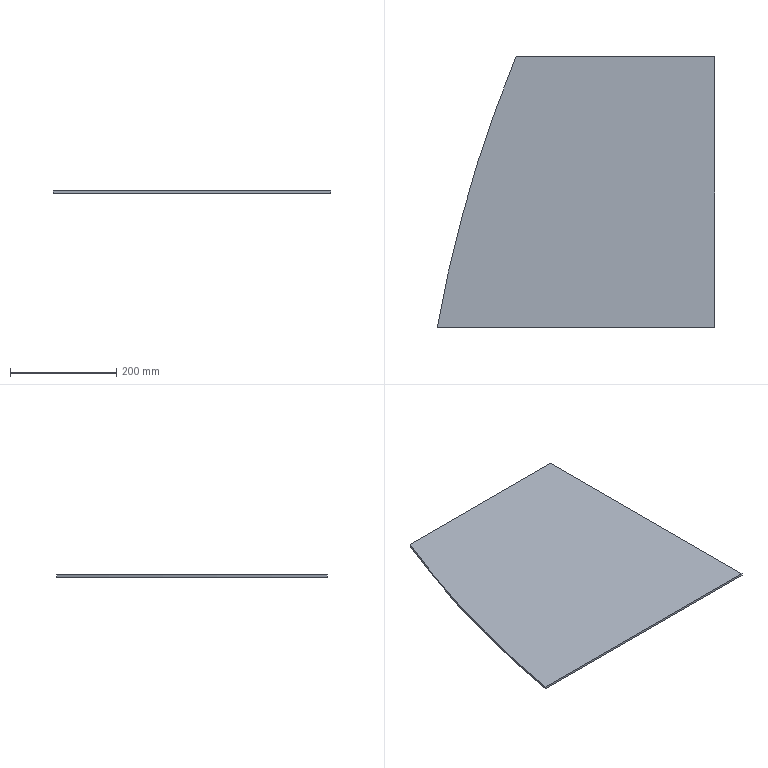Part | STEP file | 10-Side end pedal | 1 solid | 6 faces | box 521.6 x 509 x 4 mm | volume 931106 mm3 | plane 5 | cylinder 1 | commonest cylinder face diameters 4960 x1
STEP:
#1=CARTESIAN_POINT('',(0.,0.,0.));
#2=DIRECTION('',(0.,0.,1.));
#3=DIRECTION('',(1.,0.,0.));
#4=AXIS2_PLACEMENT_3D('',#1,#2,#3);
#5=CARTESIAN_POINT('',(0.,-509.,0.));
#6=VERTEX_POINT('',#5);
#7=CARTESIAN_POINT('',(0.,0.,0.));
#8=VERTEX_POINT('',#7);
#9=CARTESIAN_POINT('',(0.,0.,0.));
#10=DIRECTION('',(0.,1.,0.));
#11=VECTOR('',#10,1.);
#12=LINE('',#9,#11);
#13=CARTESIAN_POINT('',(0.,0.,4.));
#14=DIRECTION('',(-1.,0.,0.));
#15=DIRECTION('',(0.,-1.,0.));
#16=AXIS2_PLACEMENT_3D('',#13,#14,#15);
#17=PLANE('',#16);
#18=CARTESIAN_POINT('',(0.,-4.));
#19=DIRECTION('',(-1.,0.));
#20=VECTOR('',#19,1.);
#21=LINE('',#18,#20);
#22=(GEOMETRIC_REPRESENTATION_CONTEXT(2)PARAMETRIC_REPRESENTATION_CONTEXT()REPRESENTATION_CONTEXT('',''));
#23=DEFINITIONAL_REPRESENTATION('',(#21),#22);
#24=PCURVE('',#17,#23);
#25=CARTESIAN_POINT('',(1919.908,-944.243,0.));
#26=DIRECTION('',(0.,0.,1.));
#27=DIRECTION('',(1.,0.,0.));
#28=AXIS2_PLACEMENT_3D('',#25,#26,#27);
#29=PLANE('',#28);
#30=CARTESIAN_POINT('',(-1919.908,944.243));
#31=DIRECTION('',(0.,1.));
#32=VECTOR('',#31,1.);
#33=LINE('',#30,#32);
#34=(GEOMETRIC_REPRESENTATION_CONTEXT(2)PARAMETRIC_REPRESENTATION_CONTEXT()REPRESENTATION_CONTEXT('',''));
#35=DEFINITIONAL_REPRESENTATION('',(#33),#34);
#36=PCURVE('',#29,#35);
#37=SURFACE_CURVE('',#12,(#24,#36),.PCURVE_S1.);
#38=EDGE_CURVE('',#6,#8,#37,.T.);
#39=ORIENTED_EDGE('',*,*,#38,.T.);
#40=CARTESIAN_POINT('',(0.,0.,4.));
#41=VERTEX_POINT('',#40);
#42=CARTESIAN_POINT('',(0.,0.,4.));
#43=DIRECTION('',(0.,0.,-1.));
#44=VECTOR('',#43,1.);
#45=LINE('',#42,#44);
#46=CARTESIAN_POINT('',(0.,0.));
#47=DIRECTION('',(0.,-1.));
#48=VECTOR('',#47,1.);
#49=LINE('',#46,#48);
#50=(GEOMETRIC_REPRESENTATION_CONTEXT(2)PARAMETRIC_REPRESENTATION_CONTEXT()REPRESENTATION_CONTEXT('',''));
#51=DEFINITIONAL_REPRESENTATION('',(#49),#50);
#52=PCURVE('',#17,#51);
#53=CARTESIAN_POINT('',(0.,0.,4.));
#54=DIRECTION('',(0.,-1.,0.));
#55=DIRECTION('',(1.,0.,0.));
#56=AXIS2_PLACEMENT_3D('',#53,#54,#55);
#57=PLANE('',#56);
#58=CARTESIAN_POINT('',(0.,0.));
#59=DIRECTION('',(0.,-1.));
#60=VECTOR('',#59,1.);
#61=LINE('',#58,#60);
#62=(GEOMETRIC_REPRESENTATION_CONTEXT(2)PARAMETRIC_REPRESENTATION_CONTEXT()REPRESENTATION_CONTEXT('',''));
#63=DEFINITIONAL_REPRESENTATION('',(#61),#62);
#64=PCURVE('',#57,#63);
#65=SURFACE_CURVE('',#45,(#52,#64),.PCURVE_S1.);
#66=EDGE_CURVE('',#41,#8,#65,.T.);
#67=ORIENTED_EDGE('',*,*,#66,.F.);
#68=CARTESIAN_POINT('',(0.,-509.,4.));
#69=VERTEX_POINT('',#68);
#70=CARTESIAN_POINT('',(0.,0.,4.));
#71=DIRECTION('',(0.,1.,0.));
#72=VECTOR('',#71,1.);
#73=LINE('',#70,#72);
#74=CARTESIAN_POINT('',(0.,0.));
#75=DIRECTION('',(-1.,0.));
#76=VECTOR('',#75,1.);
#77=LINE('',#74,#76);
#78=(GEOMETRIC_REPRESENTATION_CONTEXT(2)PARAMETRIC_REPRESENTATION_CONTEXT()REPRESENTATION_CONTEXT('',''));
#79=DEFINITIONAL_REPRESENTATION('',(#77),#78);
#80=PCURVE('',#17,#79);
#81=CARTESIAN_POINT('',(1919.908,-944.243,4.));
#82=DIRECTION('',(0.,0.,1.));
#83=DIRECTION('',(1.,0.,0.));
#84=AXIS2_PLACEMENT_3D('',#81,#82,#83);
#85=PLANE('',#84);
#86=CARTESIAN_POINT('',(-1919.908,944.243));
#87=DIRECTION('',(0.,1.));
#88=VECTOR('',#87,1.);
#89=LINE('',#86,#88);
#90=(GEOMETRIC_REPRESENTATION_CONTEXT(2)PARAMETRIC_REPRESENTATION_CONTEXT()REPRESENTATION_CONTEXT('',''));
#91=DEFINITIONAL_REPRESENTATION('',(#89),#90);
#92=PCURVE('',#85,#91);
#93=SURFACE_CURVE('',#73,(#80,#92),.PCURVE_S1.);
#94=EDGE_CURVE('',#69,#41,#93,.T.);
#95=ORIENTED_EDGE('',*,*,#94,.F.);
#96=CARTESIAN_POINT('',(0.,-509.,4.));
#97=DIRECTION('',(0.,0.,-1.));
#98=VECTOR('',#97,1.);
#99=LINE('',#96,#98);
#100=CARTESIAN_POINT('',(509.,0.));
#101=DIRECTION('',(0.,-1.));
#102=VECTOR('',#101,1.);
#103=LINE('',#100,#102);
#104=(GEOMETRIC_REPRESENTATION_CONTEXT(2)PARAMETRIC_REPRESENTATION_CONTEXT()REPRESENTATION_CONTEXT('',''));
#105=DEFINITIONAL_REPRESENTATION('',(#103),#104);
#106=PCURVE('',#17,#105);
#107=CARTESIAN_POINT('',(0.,-509.,4.));
#108=DIRECTION('',(0.,1.,0.));
#109=DIRECTION('',(-1.,0.,0.));
#110=AXIS2_PLACEMENT_3D('',#107,#108,#109);
#111=PLANE('',#110);
#112=CARTESIAN_POINT('',(0.,0.));
#113=DIRECTION('',(0.,-1.));
#114=VECTOR('',#113,1.);
#115=LINE('',#112,#114);
#116=(GEOMETRIC_REPRESENTATION_CONTEXT(2)PARAMETRIC_REPRESENTATION_CONTEXT()REPRESENTATION_CONTEXT('',''));
#117=DEFINITIONAL_REPRESENTATION('',(#115),#116);
#118=PCURVE('',#111,#117);
#119=SURFACE_CURVE('',#99,(#106,#118),.PCURVE_S1.);
#120=EDGE_CURVE('',#69,#6,#119,.T.);
#121=ORIENTED_EDGE('',*,*,#120,.T.);
#122=EDGE_LOOP('',(#39,#67,#95,#121));
#123=FACE_BOUND('',#122,.T.);
#124=ADVANCED_FACE('',(#123),#17,.F.);
#125=CARTESIAN_POINT('',(-373.3,0.,0.));
#126=VERTEX_POINT('',#125);
#127=CARTESIAN_POINT('',(0.,0.,0.));
#128=DIRECTION('',(-1.,0.,0.));
#129=VECTOR('',#128,1.);
#130=LINE('',#127,#129);
#131=CARTESIAN_POINT('',(0.,-4.));
#132=DIRECTION('',(-1.,0.));
#133=VECTOR('',#132,1.);
#134=LINE('',#131,#133);
#135=(GEOMETRIC_REPRESENTATION_CONTEXT(2)PARAMETRIC_REPRESENTATION_CONTEXT()REPRESENTATION_CONTEXT('',''));
#136=DEFINITIONAL_REPRESENTATION('',(#134),#135);
#137=PCURVE('',#57,#136);
#138=CARTESIAN_POINT('',(-1919.908,944.243));
#139=DIRECTION('',(-1.,0.));
#140=VECTOR('',#139,1.);
#141=LINE('',#138,#140);
#142=(GEOMETRIC_REPRESENTATION_CONTEXT(2)PARAMETRIC_REPRESENTATION_CONTEXT()REPRESENTATION_CONTEXT('',''));
#143=DEFINITIONAL_REPRESENTATION('',(#141),#142);
#144=PCURVE('',#29,#143);
#145=SURFACE_CURVE('',#130,(#137,#144),.PCURVE_S1.);
#146=EDGE_CURVE('',#8,#126,#145,.T.);
#147=ORIENTED_EDGE('',*,*,#146,.T.);
#148=CARTESIAN_POINT('',(-373.3,0.,4.));
#149=VERTEX_POINT('',#148);
#150=CARTESIAN_POINT('',(-373.3,0.,4.));
#151=DIRECTION('',(0.,0.,-1.));
#152=VECTOR('',#151,1.);
#153=LINE('',#150,#152);
#154=CARTESIAN_POINT('',(-373.3,0.));
#155=DIRECTION('',(0.,-1.));
#156=VECTOR('',#155,1.);
#157=LINE('',#154,#156);
#158=(GEOMETRIC_REPRESENTATION_CONTEXT(2)PARAMETRIC_REPRESENTATION_CONTEXT()REPRESENTATION_CONTEXT('',''));
#159=DEFINITIONAL_REPRESENTATION('',(#157),#158);
#160=PCURVE('',#57,#159);
#161=CARTESIAN_POINT('',(1919.908,-944.243,4.));
#162=DIRECTION('',(0.,0.,-1.));
#163=DIRECTION('',(-1.,0.,0.));
#164=AXIS2_PLACEMENT_3D('',#161,#162,#163);
#165=CYLINDRICAL_SURFACE('',#164,2480.);
#166=CARTESIAN_POINT('',(0.3906,0.));
#167=DIRECTION('',(0.,1.));
#168=VECTOR('',#167,1.);
#169=LINE('',#166,#168);
#170=(GEOMETRIC_REPRESENTATION_CONTEXT(2)PARAMETRIC_REPRESENTATION_CONTEXT()REPRESENTATION_CONTEXT('',''));
#171=DEFINITIONAL_REPRESENTATION('',(#169),#170);
#172=PCURVE('',#165,#171);
#173=SURFACE_CURVE('',#153,(#160,#172),.PCURVE_S1.);
#174=EDGE_CURVE('',#149,#126,#173,.T.);
#175=ORIENTED_EDGE('',*,*,#174,.F.);
#176=CARTESIAN_POINT('',(0.,0.,4.));
#177=DIRECTION('',(-1.,0.,0.));
#178=VECTOR('',#177,1.);
#179=LINE('',#176,#178);
#180=CARTESIAN_POINT('',(0.,0.));
#181=DIRECTION('',(-1.,0.));
#182=VECTOR('',#181,1.);
#183=LINE('',#180,#182);
#184=(GEOMETRIC_REPRESENTATION_CONTEXT(2)PARAMETRIC_REPRESENTATION_CONTEXT()REPRESENTATION_CONTEXT('',''));
#185=DEFINITIONAL_REPRESENTATION('',(#183),#184);
#186=PCURVE('',#57,#185);
#187=CARTESIAN_POINT('',(-1919.908,944.243));
#188=DIRECTION('',(-1.,0.));
#189=VECTOR('',#188,1.);
#190=LINE('',#187,#189);
#191=(GEOMETRIC_REPRESENTATION_CONTEXT(2)PARAMETRIC_REPRESENTATION_CONTEXT()REPRESENTATION_CONTEXT('',''));
#192=DEFINITIONAL_REPRESENTATION('',(#190),#191);
#193=PCURVE('',#85,#192);
#194=SURFACE_CURVE('',#179,(#186,#193),.PCURVE_S1.);
#195=EDGE_CURVE('',#41,#149,#194,.T.);
#196=ORIENTED_EDGE('',*,*,#195,.F.);
#197=ORIENTED_EDGE('',*,*,#66,.T.);
#198=EDGE_LOOP('',(#147,#175,#196,#197));
#199=FACE_BOUND('',#198,.T.);
#200=ADVANCED_FACE('',(#199),#57,.F.);
#201=CARTESIAN_POINT('',(-521.6,-509.,0.));
#202=VERTEX_POINT('',#201);
#203=CARTESIAN_POINT('',(1919.908,-944.243,0.));
#204=DIRECTION('',(0.,0.,1.));
#205=DIRECTION('',(1.,0.,0.));
#206=AXIS2_PLACEMENT_3D('',#203,#204,#205);
#207=CIRCLE('',#206,2480.);
#208=CARTESIAN_POINT('',(3.142,4.));
#209=DIRECTION('',(-1.,0.));
#210=VECTOR('',#209,1.);
#211=LINE('',#208,#210);
#212=(GEOMETRIC_REPRESENTATION_CONTEXT(2)PARAMETRIC_REPRESENTATION_CONTEXT()REPRESENTATION_CONTEXT('',''));
#213=DEFINITIONAL_REPRESENTATION('',(#211),#212);
#214=PCURVE('',#165,#213);
#215=CARTESIAN_POINT('',(0.,0.));
#216=DIRECTION('',(1.,0.));
#217=AXIS2_PLACEMENT_2D('',#215,#216);
#218=CIRCLE('',#217,2480.);
#219=(GEOMETRIC_REPRESENTATION_CONTEXT(2)PARAMETRIC_REPRESENTATION_CONTEXT()REPRESENTATION_CONTEXT('',''));
#220=DEFINITIONAL_REPRESENTATION('',(#218),#219);
#221=PCURVE('',#29,#220);
#222=SURFACE_CURVE('',#207,(#214,#221),.PCURVE_S1.);
#223=EDGE_CURVE('',#126,#202,#222,.T.);
#224=ORIENTED_EDGE('',*,*,#223,.T.);
#225=CARTESIAN_POINT('',(-521.6,-509.,4.));
#226=VERTEX_POINT('',#225);
#227=CARTESIAN_POINT('',(-521.6,-509.,4.));
#228=DIRECTION('',(0.,0.,-1.));
#229=VECTOR('',#228,1.);
#230=LINE('',#227,#229);
#231=CARTESIAN_POINT('',(0.1764,0.));
#232=DIRECTION('',(0.,1.));
#233=VECTOR('',#232,1.);
#234=LINE('',#231,#233);
#235=(GEOMETRIC_REPRESENTATION_CONTEXT(2)PARAMETRIC_REPRESENTATION_CONTEXT()REPRESENTATION_CONTEXT('',''));
#236=DEFINITIONAL_REPRESENTATION('',(#234),#235);
#237=PCURVE('',#165,#236);
#238=CARTESIAN_POINT('',(521.6,0.));
#239=DIRECTION('',(0.,-1.));
#240=VECTOR('',#239,1.);
#241=LINE('',#238,#240);
#242=(GEOMETRIC_REPRESENTATION_CONTEXT(2)PARAMETRIC_REPRESENTATION_CONTEXT()REPRESENTATION_CONTEXT('',''));
#243=DEFINITIONAL_REPRESENTATION('',(#241),#242);
#244=PCURVE('',#111,#243);
#245=SURFACE_CURVE('',#230,(#237,#244),.PCURVE_S1.);
#246=EDGE_CURVE('',#226,#202,#245,.T.);
#247=ORIENTED_EDGE('',*,*,#246,.F.);
#248=CARTESIAN_POINT('',(1919.908,-944.243,4.));
#249=DIRECTION('',(0.,0.,1.));
#250=DIRECTION('',(1.,0.,0.));
#251=AXIS2_PLACEMENT_3D('',#248,#249,#250);
#252=CIRCLE('',#251,2480.);
#253=CARTESIAN_POINT('',(3.142,0.));
#254=DIRECTION('',(-1.,0.));
#255=VECTOR('',#254,1.);
#256=LINE('',#253,#255);
#257=(GEOMETRIC_REPRESENTATION_CONTEXT(2)PARAMETRIC_REPRESENTATION_CONTEXT()REPRESENTATION_CONTEXT('',''));
#258=DEFINITIONAL_REPRESENTATION('',(#256),#257);
#259=PCURVE('',#165,#258);
#260=CARTESIAN_POINT('',(0.,0.));
#261=DIRECTION('',(1.,0.));
#262=AXIS2_PLACEMENT_2D('',#260,#261);
#263=CIRCLE('',#262,2480.);
#264=(GEOMETRIC_REPRESENTATION_CONTEXT(2)PARAMETRIC_REPRESENTATION_CONTEXT()REPRESENTATION_CONTEXT('',''));
#265=DEFINITIONAL_REPRESENTATION('',(#263),#264);
#266=PCURVE('',#85,#265);
#267=SURFACE_CURVE('',#252,(#259,#266),.PCURVE_S1.);
#268=EDGE_CURVE('',#149,#226,#267,.T.);
#269=ORIENTED_EDGE('',*,*,#268,.F.);
#270=ORIENTED_EDGE('',*,*,#174,.T.);
#271=EDGE_LOOP('',(#224,#247,#269,#270));
#272=FACE_BOUND('',#271,.T.);
#273=ADVANCED_FACE('',(#272),#165,.T.);
#274=CARTESIAN_POINT('',(0.,-509.,0.));
#275=DIRECTION('',(1.,0.,0.));
#276=VECTOR('',#275,1.);
#277=LINE('',#274,#276);
#278=CARTESIAN_POINT('',(0.,-4.));
#279=DIRECTION('',(-1.,0.));
#280=VECTOR('',#279,1.);
#281=LINE('',#278,#280);
#282=(GEOMETRIC_REPRESENTATION_CONTEXT(2)PARAMETRIC_REPRESENTATION_CONTEXT()REPRESENTATION_CONTEXT('',''));
#283=DEFINITIONAL_REPRESENTATION('',(#281),#282);
#284=PCURVE('',#111,#283);
#285=CARTESIAN_POINT('',(-1919.908,435.243));
#286=DIRECTION('',(1.,0.));
#287=VECTOR('',#286,1.);
#288=LINE('',#285,#287);
#289=(GEOMETRIC_REPRESENTATION_CONTEXT(2)PARAMETRIC_REPRESENTATION_CONTEXT()REPRESENTATION_CONTEXT('',''));
#290=DEFINITIONAL_REPRESENTATION('',(#288),#289);
#291=PCURVE('',#29,#290);
#292=SURFACE_CURVE('',#277,(#284,#291),.PCURVE_S1.);
#293=EDGE_CURVE('',#202,#6,#292,.T.);
#294=ORIENTED_EDGE('',*,*,#293,.T.);
#295=ORIENTED_EDGE('',*,*,#120,.F.);
#296=CARTESIAN_POINT('',(0.,-509.,4.));
#297=DIRECTION('',(1.,0.,0.));
#298=VECTOR('',#297,1.);
#299=LINE('',#296,#298);
#300=CARTESIAN_POINT('',(0.,0.));
#301=DIRECTION('',(-1.,0.));
#302=VECTOR('',#301,1.);
#303=LINE('',#300,#302);
#304=(GEOMETRIC_REPRESENTATION_CONTEXT(2)PARAMETRIC_REPRESENTATION_CONTEXT()REPRESENTATION_CONTEXT('',''));
#305=DEFINITIONAL_REPRESENTATION('',(#303),#304);
#306=PCURVE('',#111,#305);
#307=CARTESIAN_POINT('',(-1919.908,435.243));
#308=DIRECTION('',(1.,0.));
#309=VECTOR('',#308,1.);
#310=LINE('',#307,#309);
#311=(GEOMETRIC_REPRESENTATION_CONTEXT(2)PARAMETRIC_REPRESENTATION_CONTEXT()REPRESENTATION_CONTEXT('',''));
#312=DEFINITIONAL_REPRESENTATION('',(#310),#311);
#313=PCURVE('',#85,#312);
#314=SURFACE_CURVE('',#299,(#306,#313),.PCURVE_S1.);
#315=EDGE_CURVE('',#226,#69,#314,.T.);
#316=ORIENTED_EDGE('',*,*,#315,.F.);
#317=ORIENTED_EDGE('',*,*,#246,.T.);
#318=EDGE_LOOP('',(#294,#295,#316,#317));
#319=FACE_BOUND('',#318,.T.);
#320=ADVANCED_FACE('',(#319),#111,.F.);
#321=ORIENTED_EDGE('',*,*,#94,.T.);
#322=ORIENTED_EDGE('',*,*,#195,.T.);
#323=ORIENTED_EDGE('',*,*,#268,.T.);
#324=ORIENTED_EDGE('',*,*,#315,.T.);
#325=EDGE_LOOP('',(#321,#322,#323,#324));
#326=FACE_BOUND('',#325,.T.);
#327=ADVANCED_FACE('',(#326),#85,.T.);
#328=ORIENTED_EDGE('',*,*,#38,.F.);
#329=ORIENTED_EDGE('',*,*,#293,.F.);
#330=ORIENTED_EDGE('',*,*,#223,.F.);
#331=ORIENTED_EDGE('',*,*,#146,.F.);
#332=EDGE_LOOP('',(#328,#329,#330,#331));
#333=FACE_BOUND('',#332,.T.);
#334=ADVANCED_FACE('',(#333),#29,.F.);
#335=CLOSED_SHELL('',(#124,#200,#273,#320,#327,#334));
#336=MANIFOLD_SOLID_BREP('',#335);
#337=(LENGTH_UNIT()NAMED_UNIT(*)SI_UNIT(.MILLI.,.METRE.));
#338=UNCERTAINTY_MEASURE_WITH_UNIT(LENGTH_MEASURE(0.0000001),#337,'','');
#339=(NAMED_UNIT(*)PLANE_ANGLE_UNIT()SI_UNIT($,.RADIAN.));
#340=(NAMED_UNIT(*)SI_UNIT($,.STERADIAN.)SOLID_ANGLE_UNIT());
#341=(GEOMETRIC_REPRESENTATION_CONTEXT(3)GLOBAL_UNCERTAINTY_ASSIGNED_CONTEXT((#338))GLOBAL_UNIT_ASSIGNED_CONTEXT((#337,#339,#340))REPRESENTATION_CONTEXT('',''));
#342=ADVANCED_BREP_SHAPE_REPRESENTATION('',(#4,#336),#341);